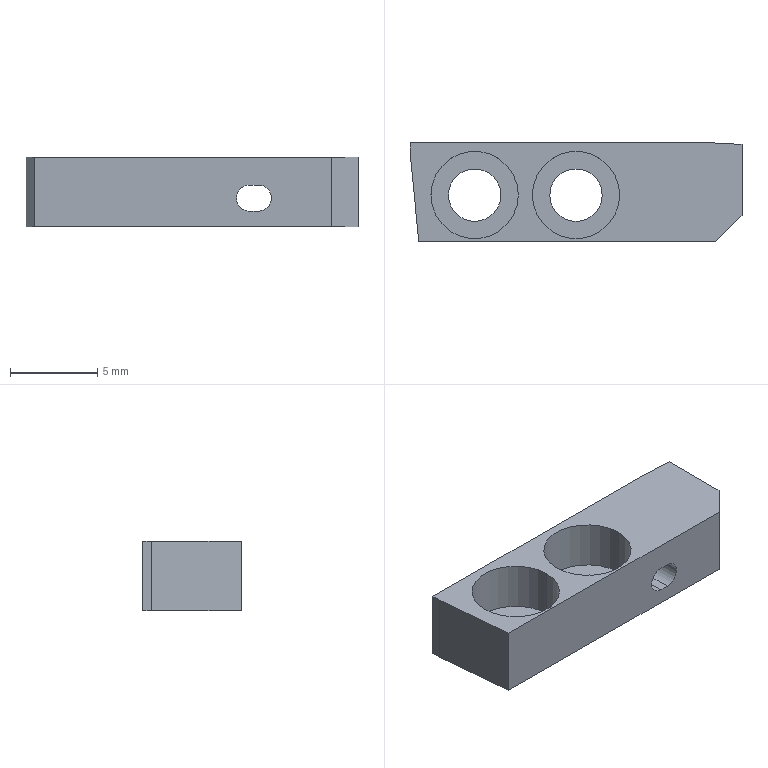Part | NX | 1 solid | 24 faces | box 19 x 5.65 x 4 mm | volume 278.189 mm3 | plane 13 | cylinder 11 | commonest cylinder face diameters 3 x4 5 x4 1.5 x3
STEP:
#1=CARTESIAN_POINT('',(1.2,2.65,4.));
#2=VERTEX_POINT('',#1);
#3=CARTESIAN_POINT('',(6.2,2.65,4.));
#4=VERTEX_POINT('',#3);
#5=CARTESIAN_POINT('',(3.7,2.65,4.));
#6=DIRECTION('',(0.,0.,1.));
#7=DIRECTION('',(1.,0.,0.));
#8=AXIS2_PLACEMENT_3D('',#5,#6,#7);
#9=CIRCLE('',#8,2.5);
#10=EDGE_CURVE('',#2,#4,#9,.T.);
#11=ORIENTED_EDGE('',*,*,#10,.T.);
#12=CARTESIAN_POINT('',(6.2,2.65,1.2));
#13=VERTEX_POINT('',#12);
#14=CARTESIAN_POINT('',(6.2,2.65,4.));
#15=DIRECTION('',(0.,0.,1.));
#16=VECTOR('',#15,1000.);
#17=LINE('',#14,#16);
#18=EDGE_CURVE('',#13,#4,#17,.T.);
#19=ORIENTED_EDGE('',*,*,#18,.F.);
#20=CARTESIAN_POINT('',(1.2,2.65,1.2));
#21=VERTEX_POINT('',#20);
#22=CARTESIAN_POINT('',(3.7,2.65,1.2));
#23=DIRECTION('',(0.,0.,1.));
#24=DIRECTION('',(1.,0.,0.));
#25=AXIS2_PLACEMENT_3D('',#22,#23,#24);
#26=CIRCLE('',#25,2.5);
#27=EDGE_CURVE('',#21,#13,#26,.T.);
#28=ORIENTED_EDGE('',*,*,#27,.F.);
#29=CARTESIAN_POINT('',(1.2,2.65,4.));
#30=DIRECTION('',(0.,0.,1.));
#31=VECTOR('',#30,1000.);
#32=LINE('',#29,#31);
#33=EDGE_CURVE('',#21,#2,#32,.T.);
#34=ORIENTED_EDGE('',*,*,#33,.T.);
#35=EDGE_LOOP('',(#11,#19,#28,#34));
#36=FACE_BOUND('',#35,.T.);
#37=CARTESIAN_POINT('',(3.7,2.65,4.));
#38=DIRECTION('',(0.,0.,1.));
#39=DIRECTION('',(1.,0.,0.));
#40=AXIS2_PLACEMENT_3D('',#37,#38,#39);
#41=CYLINDRICAL_SURFACE('',#40,2.5);
#42=ADVANCED_FACE('',(#36),#41,.F.);
#43=CARTESIAN_POINT('',(17.,5.65,0.));
#44=VERTEX_POINT('',#43);
#45=CARTESIAN_POINT('',(0.,5.65,0.));
#46=VERTEX_POINT('',#45);
#47=CARTESIAN_POINT('',(0.,5.65,0.));
#48=DIRECTION('',(-1.,0.,0.));
#49=VECTOR('',#48,1000.);
#50=LINE('',#47,#49);
#51=EDGE_CURVE('',#44,#46,#50,.T.);
#52=ORIENTED_EDGE('',*,*,#51,.T.);
#53=CARTESIAN_POINT('',(0.,5.65,4.));
#54=VERTEX_POINT('',#53);
#55=CARTESIAN_POINT('',(0.,5.65,0.));
#56=DIRECTION('',(0.,0.,1.));
#57=VECTOR('',#56,1000.);
#58=LINE('',#55,#57);
#59=EDGE_CURVE('',#46,#54,#58,.T.);
#60=ORIENTED_EDGE('',*,*,#59,.T.);
#61=CARTESIAN_POINT('',(17.,5.65,4.));
#62=VERTEX_POINT('',#61);
#63=CARTESIAN_POINT('',(0.,5.65,4.));
#64=DIRECTION('',(-1.,0.,0.));
#65=VECTOR('',#64,1000.);
#66=LINE('',#63,#65);
#67=EDGE_CURVE('',#62,#54,#66,.T.);
#68=ORIENTED_EDGE('',*,*,#67,.F.);
#69=CARTESIAN_POINT('',(17.,5.65,0.));
#70=DIRECTION('',(0.,0.,1.));
#71=VECTOR('',#70,1000.);
#72=LINE('',#69,#71);
#73=EDGE_CURVE('',#44,#62,#72,.T.);
#74=ORIENTED_EDGE('',*,*,#73,.F.);
#75=EDGE_LOOP('',(#52,#60,#68,#74));
#76=FACE_BOUND('',#75,.T.);
#77=CARTESIAN_POINT('',(12.8,5.65,0.9));
#78=VERTEX_POINT('',#77);
#79=CARTESIAN_POINT('',(13.3,5.65,0.9));
#80=VERTEX_POINT('',#79);
#81=CARTESIAN_POINT('',(0.,5.65,0.9));
#82=DIRECTION('',(1.,0.,0.));
#83=VECTOR('',#82,1000.);
#84=LINE('',#81,#83);
#85=EDGE_CURVE('',#78,#80,#84,.T.);
#86=ORIENTED_EDGE('',*,*,#85,.T.);
#87=CARTESIAN_POINT('',(13.3,5.65,2.4));
#88=VERTEX_POINT('',#87);
#89=CARTESIAN_POINT('',(13.3,5.65,1.65));
#90=DIRECTION('',(0.,1.,0.));
#91=DIRECTION('',(-1.,0.,0.));
#92=AXIS2_PLACEMENT_3D('',#89,#90,#91);
#93=CIRCLE('',#92,0.75);
#94=EDGE_CURVE('',#88,#80,#93,.T.);
#95=ORIENTED_EDGE('',*,*,#94,.F.);
#96=CARTESIAN_POINT('',(12.8,5.65,2.4));
#97=VERTEX_POINT('',#96);
#98=CARTESIAN_POINT('',(0.,5.65,2.4));
#99=DIRECTION('',(-1.,0.,0.));
#100=VECTOR('',#99,1000.);
#101=LINE('',#98,#100);
#102=EDGE_CURVE('',#88,#97,#101,.T.);
#103=ORIENTED_EDGE('',*,*,#102,.T.);
#104=CARTESIAN_POINT('',(12.05,5.65,1.65));
#105=VERTEX_POINT('',#104);
#106=CARTESIAN_POINT('',(12.8,5.65,1.65));
#107=DIRECTION('',(0.,1.,0.));
#108=DIRECTION('',(-1.,0.,0.));
#109=AXIS2_PLACEMENT_3D('',#106,#107,#108);
#110=CIRCLE('',#109,0.75);
#111=EDGE_CURVE('',#105,#97,#110,.T.);
#112=ORIENTED_EDGE('',*,*,#111,.F.);
#113=CARTESIAN_POINT('',(12.8,5.65,1.65));
#114=DIRECTION('',(0.,1.,0.));
#115=DIRECTION('',(-1.,0.,0.));
#116=AXIS2_PLACEMENT_3D('',#113,#114,#115);
#117=CIRCLE('',#116,0.75);
#118=EDGE_CURVE('',#78,#105,#117,.T.);
#119=ORIENTED_EDGE('',*,*,#118,.F.);
#120=EDGE_LOOP('',(#86,#95,#103,#112,#119));
#121=FACE_BOUND('',#120,.T.);
#122=CARTESIAN_POINT('',(19.,5.65,0.));
#123=DIRECTION('',(0.,1.,0.));
#124=DIRECTION('',(1.,0.,0.));
#125=AXIS2_PLACEMENT_3D('',#122,#123,#124);
#126=PLANE('',#125);
#127=ADVANCED_FACE('',(#76,#121),#126,.T.);
#128=CARTESIAN_POINT('',(0.,5.15,4.));
#129=VERTEX_POINT('',#128);
#130=CARTESIAN_POINT('',(0.,5.15,0.));
#131=VERTEX_POINT('',#130);
#132=CARTESIAN_POINT('',(0.,5.15,0.));
#133=DIRECTION('',(0.,0.,-1.));
#134=VECTOR('',#133,1000.);
#135=LINE('',#132,#134);
#136=EDGE_CURVE('',#129,#131,#135,.T.);
#137=ORIENTED_EDGE('',*,*,#136,.F.);
#138=CARTESIAN_POINT('',(0.,0.,4.));
#139=DIRECTION('',(0.,-1.,0.));
#140=VECTOR('',#139,1000.);
#141=LINE('',#138,#140);
#142=EDGE_CURVE('',#54,#129,#141,.T.);
#143=ORIENTED_EDGE('',*,*,#142,.F.);
#144=ORIENTED_EDGE('',*,*,#59,.F.);
#145=CARTESIAN_POINT('',(0.,0.,0.));
#146=DIRECTION('',(0.,-1.,0.));
#147=VECTOR('',#146,1000.);
#148=LINE('',#145,#147);
#149=EDGE_CURVE('',#46,#131,#148,.T.);
#150=ORIENTED_EDGE('',*,*,#149,.T.);
#151=EDGE_LOOP('',(#137,#143,#144,#150));
#152=FACE_BOUND('',#151,.T.);
#153=CARTESIAN_POINT('',(0.,5.65,0.));
#154=DIRECTION('',(-1.,0.,0.));
#155=DIRECTION('',(0.,0.,1.));
#156=AXIS2_PLACEMENT_3D('',#153,#154,#155);
#157=PLANE('',#156);
#158=ADVANCED_FACE('',(#152),#157,.T.);
#159=CARTESIAN_POINT('',(12.,2.65,1.2));
#160=VERTEX_POINT('',#159);
#161=CARTESIAN_POINT('',(7.,2.65,1.2));
#162=VERTEX_POINT('',#161);
#163=CARTESIAN_POINT('',(9.5,2.65,1.2));
#164=DIRECTION('',(0.,0.,1.));
#165=DIRECTION('',(-1.,0.,0.));
#166=AXIS2_PLACEMENT_3D('',#163,#164,#165);
#167=CIRCLE('',#166,2.5);
#168=EDGE_CURVE('',#160,#162,#167,.T.);
#169=ORIENTED_EDGE('',*,*,#168,.T.);
#170=CARTESIAN_POINT('',(9.5,2.65,1.2));
#171=DIRECTION('',(0.,0.,1.));
#172=DIRECTION('',(-1.,0.,0.));
#173=AXIS2_PLACEMENT_3D('',#170,#171,#172);
#174=CIRCLE('',#173,2.5);
#175=EDGE_CURVE('',#162,#160,#174,.T.);
#176=ORIENTED_EDGE('',*,*,#175,.T.);
#177=EDGE_LOOP('',(#169,#176));
#178=FACE_BOUND('',#177,.T.);
#179=CARTESIAN_POINT('',(11.,2.65,1.2));
#180=VERTEX_POINT('',#179);
#181=CARTESIAN_POINT('',(8.,2.65,1.2));
#182=VERTEX_POINT('',#181);
#183=CARTESIAN_POINT('',(9.5,2.65,1.2));
#184=DIRECTION('',(0.,0.,1.));
#185=DIRECTION('',(-1.,0.,0.));
#186=AXIS2_PLACEMENT_3D('',#183,#184,#185);
#187=CIRCLE('',#186,1.5);
#188=EDGE_CURVE('',#180,#182,#187,.T.);
#189=ORIENTED_EDGE('',*,*,#188,.F.);
#190=CARTESIAN_POINT('',(9.5,2.65,1.2));
#191=DIRECTION('',(0.,0.,1.));
#192=DIRECTION('',(-1.,0.,0.));
#193=AXIS2_PLACEMENT_3D('',#190,#191,#192);
#194=CIRCLE('',#193,1.5);
#195=EDGE_CURVE('',#182,#180,#194,.T.);
#196=ORIENTED_EDGE('',*,*,#195,.F.);
#197=EDGE_LOOP('',(#189,#196));
#198=FACE_BOUND('',#197,.T.);
#199=CARTESIAN_POINT('',(9.5,2.65,1.2));
#200=DIRECTION('',(0.,0.,1.));
#201=DIRECTION('',(1.,0.,0.));
#202=AXIS2_PLACEMENT_3D('',#199,#200,#201);
#203=PLANE('',#202);
#204=ADVANCED_FACE('',(#178,#198),#203,.T.);
#205=ORIENTED_EDGE('',*,*,#73,.T.);
#206=CARTESIAN_POINT('',(19.,5.545,4.));
#207=VERTEX_POINT('',#206);
#208=CARTESIAN_POINT('',(0.,6.541,4.));
#209=DIRECTION('',(-0.9986,0.05234,0.));
#210=VECTOR('',#209,1000.);
#211=LINE('',#208,#210);
#212=EDGE_CURVE('',#207,#62,#211,.T.);
#213=ORIENTED_EDGE('',*,*,#212,.F.);
#214=CARTESIAN_POINT('',(19.,5.545,0.));
#215=VERTEX_POINT('',#214);
#216=CARTESIAN_POINT('',(19.,5.545,0.));
#217=DIRECTION('',(0.,0.,-1.));
#218=VECTOR('',#217,1000.);
#219=LINE('',#216,#218);
#220=EDGE_CURVE('',#207,#215,#219,.T.);
#221=ORIENTED_EDGE('',*,*,#220,.T.);
#222=CARTESIAN_POINT('',(0.,6.541,0.));
#223=DIRECTION('',(-0.9986,0.05234,0.));
#224=VECTOR('',#223,1000.);
#225=LINE('',#222,#224);
#226=EDGE_CURVE('',#215,#44,#225,.T.);
#227=ORIENTED_EDGE('',*,*,#226,.T.);
#228=EDGE_LOOP('',(#205,#213,#221,#227));
#229=FACE_BOUND('',#228,.T.);
#230=CARTESIAN_POINT('',(17.,5.65,0.));
#231=DIRECTION('',(0.05234,0.9986,0.));
#232=DIRECTION('',(0.,0.,-1.));
#233=AXIS2_PLACEMENT_3D('',#230,#231,#232);
#234=PLANE('',#233);
#235=ADVANCED_FACE('',(#229),#234,.T.);
#236=CARTESIAN_POINT('',(19.,1.5,0.));
#237=VERTEX_POINT('',#236);
#238=CARTESIAN_POINT('',(19.,0.,0.));
#239=DIRECTION('',(0.,1.,0.));
#240=VECTOR('',#239,1000.);
#241=LINE('',#238,#240);
#242=EDGE_CURVE('',#237,#215,#241,.T.);
#243=ORIENTED_EDGE('',*,*,#242,.T.);
#244=ORIENTED_EDGE('',*,*,#220,.F.);
#245=CARTESIAN_POINT('',(19.,1.5,4.));
#246=VERTEX_POINT('',#245);
#247=CARTESIAN_POINT('',(19.,0.,4.));
#248=DIRECTION('',(0.,1.,0.));
#249=VECTOR('',#248,1000.);
#250=LINE('',#247,#249);
#251=EDGE_CURVE('',#246,#207,#250,.T.);
#252=ORIENTED_EDGE('',*,*,#251,.F.);
#253=CARTESIAN_POINT('',(19.,1.5,0.));
#254=DIRECTION('',(0.,0.,1.));
#255=VECTOR('',#254,1000.);
#256=LINE('',#253,#255);
#257=EDGE_CURVE('',#237,#246,#256,.T.);
#258=ORIENTED_EDGE('',*,*,#257,.F.);
#259=EDGE_LOOP('',(#243,#244,#252,#258));
#260=FACE_BOUND('',#259,.T.);
#261=CARTESIAN_POINT('',(19.,0.,0.));
#262=DIRECTION('',(1.,0.,0.));
#263=DIRECTION('',(0.,1.,0.));
#264=AXIS2_PLACEMENT_3D('',#261,#262,#263);
#265=PLANE('',#264);
#266=ADVANCED_FACE('',(#260),#265,.T.);
#267=ORIENTED_EDGE('',*,*,#257,.T.);
#268=CARTESIAN_POINT('',(17.5,0.,4.));
#269=VERTEX_POINT('',#268);
#270=CARTESIAN_POINT('',(17.5,0.,4.));
#271=DIRECTION('',(0.7071,0.7071,0.));
#272=VECTOR('',#271,1000.);
#273=LINE('',#270,#272);
#274=EDGE_CURVE('',#269,#246,#273,.T.);
#275=ORIENTED_EDGE('',*,*,#274,.F.);
#276=CARTESIAN_POINT('',(17.5,0.,0.));
#277=VERTEX_POINT('',#276);
#278=CARTESIAN_POINT('',(17.5,0.,0.));
#279=DIRECTION('',(0.,0.,1.));
#280=VECTOR('',#279,1000.);
#281=LINE('',#278,#280);
#282=EDGE_CURVE('',#277,#269,#281,.T.);
#283=ORIENTED_EDGE('',*,*,#282,.F.);
#284=CARTESIAN_POINT('',(17.5,0.,0.));
#285=DIRECTION('',(0.7071,0.7071,0.));
#286=VECTOR('',#285,1000.);
#287=LINE('',#284,#286);
#288=EDGE_CURVE('',#277,#237,#287,.T.);
#289=ORIENTED_EDGE('',*,*,#288,.T.);
#290=EDGE_LOOP('',(#267,#275,#283,#289));
#291=FACE_BOUND('',#290,.T.);
#292=CARTESIAN_POINT('',(19.,1.5,0.));
#293=DIRECTION('',(0.7071,-0.7071,0.));
#294=DIRECTION('',(0.,0.,-1.));
#295=AXIS2_PLACEMENT_3D('',#292,#293,#294);
#296=PLANE('',#295);
#297=ADVANCED_FACE('',(#291),#296,.T.);
#298=CARTESIAN_POINT('',(3.7,2.65,1.2));
#299=DIRECTION('',(0.,0.,1.));
#300=DIRECTION('',(1.,0.,0.));
#301=AXIS2_PLACEMENT_3D('',#298,#299,#300);
#302=CIRCLE('',#301,2.5);
#303=EDGE_CURVE('',#13,#21,#302,.T.);
#304=ORIENTED_EDGE('',*,*,#303,.T.);
#305=ORIENTED_EDGE('',*,*,#27,.T.);
#306=EDGE_LOOP('',(#304,#305));
#307=FACE_BOUND('',#306,.T.);
#308=CARTESIAN_POINT('',(5.2,2.65,1.2));
#309=VERTEX_POINT('',#308);
#310=CARTESIAN_POINT('',(2.2,2.65,1.2));
#311=VERTEX_POINT('',#310);
#312=CARTESIAN_POINT('',(3.7,2.65,1.2));
#313=DIRECTION('',(0.,0.,1.));
#314=DIRECTION('',(-1.,0.,0.));
#315=AXIS2_PLACEMENT_3D('',#312,#313,#314);
#316=CIRCLE('',#315,1.5);
#317=EDGE_CURVE('',#309,#311,#316,.T.);
#318=ORIENTED_EDGE('',*,*,#317,.F.);
#319=CARTESIAN_POINT('',(3.7,2.65,1.2));
#320=DIRECTION('',(0.,0.,1.));
#321=DIRECTION('',(-1.,0.,0.));
#322=AXIS2_PLACEMENT_3D('',#319,#320,#321);
#323=CIRCLE('',#322,1.5);
#324=EDGE_CURVE('',#311,#309,#323,.T.);
#325=ORIENTED_EDGE('',*,*,#324,.F.);
#326=EDGE_LOOP('',(#318,#325));
#327=FACE_BOUND('',#326,.T.);
#328=CARTESIAN_POINT('',(8.521,3.606,1.2));
#329=DIRECTION('',(0.,0.,1.));
#330=DIRECTION('',(1.,0.,0.));
#331=AXIS2_PLACEMENT_3D('',#328,#329,#330);
#332=PLANE('',#331);
#333=ADVANCED_FACE('',(#307,#327),#332,.T.);
#334=CARTESIAN_POINT('',(12.,2.65,4.));
#335=VERTEX_POINT('',#334);
#336=CARTESIAN_POINT('',(7.,2.65,4.));
#337=VERTEX_POINT('',#336);
#338=CARTESIAN_POINT('',(9.5,2.65,4.));
#339=DIRECTION('',(0.,0.,1.));
#340=DIRECTION('',(-1.,0.,0.));
#341=AXIS2_PLACEMENT_3D('',#338,#339,#340);
#342=CIRCLE('',#341,2.5);
#343=EDGE_CURVE('',#335,#337,#342,.T.);
#344=ORIENTED_EDGE('',*,*,#343,.T.);
#345=CARTESIAN_POINT('',(7.,2.65,-0.62));
#346=DIRECTION('',(0.,0.,1.));
#347=VECTOR('',#346,1000.);
#348=LINE('',#345,#347);
#349=EDGE_CURVE('',#337,#162,#348,.F.);
#350=ORIENTED_EDGE('',*,*,#349,.T.);
#351=ORIENTED_EDGE('',*,*,#168,.F.);
#352=CARTESIAN_POINT('',(12.,2.65,-0.62));
#353=DIRECTION('',(0.,0.,1.));
#354=VECTOR('',#353,1000.);
#355=LINE('',#352,#354);
#356=EDGE_CURVE('',#335,#160,#355,.F.);
#357=ORIENTED_EDGE('',*,*,#356,.F.);
#358=EDGE_LOOP('',(#344,#350,#351,#357));
#359=FACE_BOUND('',#358,.T.);
#360=CARTESIAN_POINT('',(9.5,2.65,-0.62));
#361=DIRECTION('',(0.,0.,1.));
#362=DIRECTION('',(-1.,0.,0.));
#363=AXIS2_PLACEMENT_3D('',#360,#361,#362);
#364=CYLINDRICAL_SURFACE('',#363,2.5);
#365=ADVANCED_FACE('',(#359),#364,.F.);
#366=ORIENTED_EDGE('',*,*,#317,.T.);
#367=CARTESIAN_POINT('',(2.2,2.65,0.));
#368=VERTEX_POINT('',#367);
#369=CARTESIAN_POINT('',(2.2,2.65,-0.62));
#370=DIRECTION('',(0.,0.,1.));
#371=VECTOR('',#370,1000.);
#372=LINE('',#369,#371);
#373=EDGE_CURVE('',#311,#368,#372,.F.);
#374=ORIENTED_EDGE('',*,*,#373,.T.);
#375=CARTESIAN_POINT('',(5.2,2.65,0.));
#376=VERTEX_POINT('',#375);
#377=CARTESIAN_POINT('',(3.7,2.65,0.));
#378=DIRECTION('',(0.,0.,1.));
#379=DIRECTION('',(-1.,0.,0.));
#380=AXIS2_PLACEMENT_3D('',#377,#378,#379);
#381=CIRCLE('',#380,1.5);
#382=EDGE_CURVE('',#376,#368,#381,.T.);
#383=ORIENTED_EDGE('',*,*,#382,.F.);
#384=CARTESIAN_POINT('',(5.2,2.65,-0.62));
#385=DIRECTION('',(0.,0.,1.));
#386=VECTOR('',#385,1000.);
#387=LINE('',#384,#386);
#388=EDGE_CURVE('',#309,#376,#387,.F.);
#389=ORIENTED_EDGE('',*,*,#388,.F.);
#390=EDGE_LOOP('',(#366,#374,#383,#389));
#391=FACE_BOUND('',#390,.T.);
#392=CARTESIAN_POINT('',(3.7,2.65,-0.62));
#393=DIRECTION('',(0.,0.,1.));
#394=DIRECTION('',(-1.,0.,0.));
#395=AXIS2_PLACEMENT_3D('',#392,#393,#394);
#396=CYLINDRICAL_SURFACE('',#395,1.5);
#397=ADVANCED_FACE('',(#391),#396,.F.);
#398=ORIENTED_EDGE('',*,*,#149,.F.);
#399=ORIENTED_EDGE('',*,*,#51,.F.);
#400=ORIENTED_EDGE('',*,*,#226,.F.);
#401=ORIENTED_EDGE('',*,*,#242,.F.);
#402=ORIENTED_EDGE('',*,*,#288,.F.);
#403=CARTESIAN_POINT('',(0.5,0.,0.));
#404=VERTEX_POINT('',#403);
#405=CARTESIAN_POINT('',(0.,0.,0.));
#406=DIRECTION('',(1.,0.,0.));
#407=VECTOR('',#406,1000.);
#408=LINE('',#405,#407);
#409=EDGE_CURVE('',#404,#277,#408,.T.);
#410=ORIENTED_EDGE('',*,*,#409,.F.);
#411=CARTESIAN_POINT('',(0.5,0.,0.));
#412=DIRECTION('',(-0.09663,0.9953,0.));
#413=VECTOR('',#412,1000.);
#414=LINE('',#411,#413);
#415=EDGE_CURVE('',#404,#131,#414,.T.);
#416=ORIENTED_EDGE('',*,*,#415,.T.);
#417=EDGE_LOOP('',(#398,#399,#400,#401,#402,#410,#416));
#418=FACE_BOUND('',#417,.T.);
#419=CARTESIAN_POINT('',(11.,2.65,0.));
#420=VERTEX_POINT('',#419);
#421=CARTESIAN_POINT('',(8.,2.65,0.));
#422=VERTEX_POINT('',#421);
#423=CARTESIAN_POINT('',(9.5,2.65,0.));
#424=DIRECTION('',(0.,0.,1.));
#425=DIRECTION('',(-1.,0.,0.));
#426=AXIS2_PLACEMENT_3D('',#423,#424,#425);
#427=CIRCLE('',#426,1.5);
#428=EDGE_CURVE('',#420,#422,#427,.T.);
#429=ORIENTED_EDGE('',*,*,#428,.T.);
#430=CARTESIAN_POINT('',(9.5,2.65,0.));
#431=DIRECTION('',(0.,0.,1.));
#432=DIRECTION('',(-1.,0.,0.));
#433=AXIS2_PLACEMENT_3D('',#430,#431,#432);
#434=CIRCLE('',#433,1.5);
#435=EDGE_CURVE('',#422,#420,#434,.T.);
#436=ORIENTED_EDGE('',*,*,#435,.T.);
#437=EDGE_LOOP('',(#429,#436));
#438=FACE_BOUND('',#437,.T.);
#439=CARTESIAN_POINT('',(3.7,2.65,0.));
#440=DIRECTION('',(0.,0.,1.));
#441=DIRECTION('',(-1.,0.,0.));
#442=AXIS2_PLACEMENT_3D('',#439,#440,#441);
#443=CIRCLE('',#442,1.5);
#444=EDGE_CURVE('',#368,#376,#443,.T.);
#445=ORIENTED_EDGE('',*,*,#444,.T.);
#446=ORIENTED_EDGE('',*,*,#382,.T.);
#447=EDGE_LOOP('',(#445,#446));
#448=FACE_BOUND('',#447,.T.);
#449=CARTESIAN_POINT('',(0.,0.,0.));
#450=DIRECTION('',(0.,0.,1.));
#451=DIRECTION('',(1.,0.,0.));
#452=AXIS2_PLACEMENT_3D('',#449,#450,#451);
#453=PLANE('',#452);
#454=ADVANCED_FACE('',(#418,#438,#448),#453,.F.);
#455=ORIENTED_EDGE('',*,*,#188,.T.);
#456=CARTESIAN_POINT('',(8.,2.65,-0.62));
#457=DIRECTION('',(0.,0.,1.));
#458=VECTOR('',#457,1000.);
#459=LINE('',#456,#458);
#460=EDGE_CURVE('',#182,#422,#459,.F.);
#461=ORIENTED_EDGE('',*,*,#460,.T.);
#462=ORIENTED_EDGE('',*,*,#428,.F.);
#463=CARTESIAN_POINT('',(11.,2.65,-0.62));
#464=DIRECTION('',(0.,0.,1.));
#465=VECTOR('',#464,1000.);
#466=LINE('',#463,#465);
#467=EDGE_CURVE('',#180,#420,#466,.F.);
#468=ORIENTED_EDGE('',*,*,#467,.F.);
#469=EDGE_LOOP('',(#455,#461,#462,#468));
#470=FACE_BOUND('',#469,.T.);
#471=CARTESIAN_POINT('',(9.5,2.65,-0.62));
#472=DIRECTION('',(0.,0.,1.));
#473=DIRECTION('',(-1.,0.,0.));
#474=AXIS2_PLACEMENT_3D('',#471,#472,#473);
#475=CYLINDRICAL_SURFACE('',#474,1.5);
#476=ADVANCED_FACE('',(#470),#475,.F.);
#477=CARTESIAN_POINT('',(0.5,0.,4.));
#478=VERTEX_POINT('',#477);
#479=CARTESIAN_POINT('',(0.,0.,4.));
#480=DIRECTION('',(-1.,0.,0.));
#481=VECTOR('',#480,1000.);
#482=LINE('',#479,#481);
#483=EDGE_CURVE('',#269,#478,#482,.T.);
#484=ORIENTED_EDGE('',*,*,#483,.F.);
#485=ORIENTED_EDGE('',*,*,#274,.T.);
#486=ORIENTED_EDGE('',*,*,#251,.T.);
#487=ORIENTED_EDGE('',*,*,#212,.T.);
#488=ORIENTED_EDGE('',*,*,#67,.T.);
#489=ORIENTED_EDGE('',*,*,#142,.T.);
#490=CARTESIAN_POINT('',(0.5,0.,4.));
#491=DIRECTION('',(-0.09663,0.9953,0.));
#492=VECTOR('',#491,1000.);
#493=LINE('',#490,#492);
#494=EDGE_CURVE('',#478,#129,#493,.T.);
#495=ORIENTED_EDGE('',*,*,#494,.F.);
#496=EDGE_LOOP('',(#484,#485,#486,#487,#488,#489,#495));
#497=FACE_BOUND('',#496,.T.);
#498=ORIENTED_EDGE('',*,*,#343,.F.);
#499=CARTESIAN_POINT('',(9.5,2.65,4.));
#500=DIRECTION('',(0.,0.,1.));
#501=DIRECTION('',(-1.,0.,0.));
#502=AXIS2_PLACEMENT_3D('',#499,#500,#501);
#503=CIRCLE('',#502,2.5);
#504=EDGE_CURVE('',#337,#335,#503,.T.);
#505=ORIENTED_EDGE('',*,*,#504,.F.);
#506=EDGE_LOOP('',(#498,#505));
#507=FACE_BOUND('',#506,.T.);
#508=ORIENTED_EDGE('',*,*,#10,.F.);
#509=CARTESIAN_POINT('',(3.7,2.65,4.));
#510=DIRECTION('',(0.,0.,1.));
#511=DIRECTION('',(1.,0.,0.));
#512=AXIS2_PLACEMENT_3D('',#509,#510,#511);
#513=CIRCLE('',#512,2.5);
#514=EDGE_CURVE('',#4,#2,#513,.T.);
#515=ORIENTED_EDGE('',*,*,#514,.F.);
#516=EDGE_LOOP('',(#508,#515));
#517=FACE_BOUND('',#516,.T.);
#518=CARTESIAN_POINT('',(0.,0.,4.));
#519=DIRECTION('',(0.,0.,1.));
#520=DIRECTION('',(1.,0.,0.));
#521=AXIS2_PLACEMENT_3D('',#518,#519,#520);
#522=PLANE('',#521);
#523=ADVANCED_FACE('',(#497,#507,#517),#522,.T.);
#524=CARTESIAN_POINT('',(0.5,0.,0.));
#525=DIRECTION('',(0.,0.,1.));
#526=VECTOR('',#525,1000.);
#527=LINE('',#524,#526);
#528=EDGE_CURVE('',#404,#478,#527,.T.);
#529=ORIENTED_EDGE('',*,*,#528,.F.);
#530=ORIENTED_EDGE('',*,*,#409,.T.);
#531=ORIENTED_EDGE('',*,*,#282,.T.);
#532=ORIENTED_EDGE('',*,*,#483,.T.);
#533=EDGE_LOOP('',(#529,#530,#531,#532));
#534=FACE_BOUND('',#533,.T.);
#535=CARTESIAN_POINT('',(13.3,0.,0.9));
#536=VERTEX_POINT('',#535);
#537=CARTESIAN_POINT('',(12.8,0.,0.9));
#538=VERTEX_POINT('',#537);
#539=CARTESIAN_POINT('',(0.,0.,0.9));
#540=DIRECTION('',(-1.,0.,0.));
#541=VECTOR('',#540,1000.);
#542=LINE('',#539,#541);
#543=EDGE_CURVE('',#536,#538,#542,.T.);
#544=ORIENTED_EDGE('',*,*,#543,.T.);
#545=CARTESIAN_POINT('',(12.05,0.,1.65));
#546=VERTEX_POINT('',#545);
#547=CARTESIAN_POINT('',(12.8,0.,1.65));
#548=DIRECTION('',(0.,1.,0.));
#549=DIRECTION('',(-1.,0.,0.));
#550=AXIS2_PLACEMENT_3D('',#547,#548,#549);
#551=CIRCLE('',#550,0.75);
#552=EDGE_CURVE('',#538,#546,#551,.T.);
#553=ORIENTED_EDGE('',*,*,#552,.T.);
#554=CARTESIAN_POINT('',(12.8,0.,2.4));
#555=VERTEX_POINT('',#554);
#556=CARTESIAN_POINT('',(12.8,0.,1.65));
#557=DIRECTION('',(0.,1.,0.));
#558=DIRECTION('',(-1.,0.,0.));
#559=AXIS2_PLACEMENT_3D('',#556,#557,#558);
#560=CIRCLE('',#559,0.75);
#561=EDGE_CURVE('',#546,#555,#560,.T.);
#562=ORIENTED_EDGE('',*,*,#561,.T.);
#563=CARTESIAN_POINT('',(13.3,0.,2.4));
#564=VERTEX_POINT('',#563);
#565=CARTESIAN_POINT('',(0.,0.,2.4));
#566=DIRECTION('',(1.,0.,0.));
#567=VECTOR('',#566,1000.);
#568=LINE('',#565,#567);
#569=EDGE_CURVE('',#555,#564,#568,.T.);
#570=ORIENTED_EDGE('',*,*,#569,.T.);
#571=CARTESIAN_POINT('',(13.3,0.,1.65));
#572=DIRECTION('',(0.,1.,0.));
#573=DIRECTION('',(-1.,0.,0.));
#574=AXIS2_PLACEMENT_3D('',#571,#572,#573);
#575=CIRCLE('',#574,0.75);
#576=EDGE_CURVE('',#564,#536,#575,.T.);
#577=ORIENTED_EDGE('',*,*,#576,.T.);
#578=EDGE_LOOP('',(#544,#553,#562,#570,#577));
#579=FACE_BOUND('',#578,.T.);
#580=CARTESIAN_POINT('',(0.,0.,0.));
#581=DIRECTION('',(0.,-1.,0.));
#582=DIRECTION('',(0.,0.,-1.));
#583=AXIS2_PLACEMENT_3D('',#580,#581,#582);
#584=PLANE('',#583);
#585=ADVANCED_FACE('',(#534,#579),#584,.T.);
#586=ORIENTED_EDGE('',*,*,#543,.F.);
#587=CARTESIAN_POINT('',(13.3,-0.5652,0.9));
#588=DIRECTION('',(0.,1.,0.));
#589=VECTOR('',#588,1000.);
#590=LINE('',#587,#589);
#591=EDGE_CURVE('',#536,#80,#590,.T.);
#592=ORIENTED_EDGE('',*,*,#591,.T.);
#593=ORIENTED_EDGE('',*,*,#85,.F.);
#594=CARTESIAN_POINT('',(12.8,-0.5652,0.9));
#595=DIRECTION('',(0.,1.,0.));
#596=VECTOR('',#595,1000.);
#597=LINE('',#594,#596);
#598=EDGE_CURVE('',#538,#78,#597,.T.);
#599=ORIENTED_EDGE('',*,*,#598,.F.);
#600=EDGE_LOOP('',(#586,#592,#593,#599));
#601=FACE_BOUND('',#600,.T.);
#602=CARTESIAN_POINT('',(12.8,-0.5652,0.9));
#603=DIRECTION('',(0.,0.,-1.));
#604=DIRECTION('',(0.,-1.,0.));
#605=AXIS2_PLACEMENT_3D('',#602,#603,#604);
#606=PLANE('',#605);
#607=ADVANCED_FACE('',(#601),#606,.F.);
#608=CARTESIAN_POINT('',(12.05,-0.5652,1.65));
#609=DIRECTION('',(0.,1.,0.));
#610=VECTOR('',#609,1000.);
#611=LINE('',#608,#610);
#612=EDGE_CURVE('',#546,#105,#611,.T.);
#613=ORIENTED_EDGE('',*,*,#612,.F.);
#614=ORIENTED_EDGE('',*,*,#552,.F.);
#615=ORIENTED_EDGE('',*,*,#598,.T.);
#616=ORIENTED_EDGE('',*,*,#118,.T.);
#617=EDGE_LOOP('',(#613,#614,#615,#616));
#618=FACE_BOUND('',#617,.T.);
#619=CARTESIAN_POINT('',(12.8,-0.5652,1.65));
#620=DIRECTION('',(0.,1.,0.));
#621=DIRECTION('',(-1.,0.,0.));
#622=AXIS2_PLACEMENT_3D('',#619,#620,#621);
#623=CYLINDRICAL_SURFACE('',#622,0.75);
#624=ADVANCED_FACE('',(#618),#623,.F.);
#625=ORIENTED_EDGE('',*,*,#102,.F.);
#626=CARTESIAN_POINT('',(13.3,-0.5652,2.4));
#627=DIRECTION('',(0.,1.,0.));
#628=VECTOR('',#627,1000.);
#629=LINE('',#626,#628);
#630=EDGE_CURVE('',#564,#88,#629,.T.);
#631=ORIENTED_EDGE('',*,*,#630,.F.);
#632=ORIENTED_EDGE('',*,*,#569,.F.);
#633=CARTESIAN_POINT('',(12.8,-0.5652,2.4));
#634=DIRECTION('',(0.,1.,0.));
#635=VECTOR('',#634,1000.);
#636=LINE('',#633,#635);
#637=EDGE_CURVE('',#555,#97,#636,.T.);
#638=ORIENTED_EDGE('',*,*,#637,.T.);
#639=EDGE_LOOP('',(#625,#631,#632,#638));
#640=FACE_BOUND('',#639,.T.);
#641=CARTESIAN_POINT('',(13.3,-0.5652,2.4));
#642=DIRECTION('',(0.,0.,1.));
#643=DIRECTION('',(1.,0.,0.));
#644=AXIS2_PLACEMENT_3D('',#641,#642,#643);
#645=PLANE('',#644);
#646=ADVANCED_FACE('',(#640),#645,.F.);
#647=ORIENTED_EDGE('',*,*,#576,.F.);
#648=ORIENTED_EDGE('',*,*,#630,.T.);
#649=ORIENTED_EDGE('',*,*,#94,.T.);
#650=ORIENTED_EDGE('',*,*,#591,.F.);
#651=EDGE_LOOP('',(#647,#648,#649,#650));
#652=FACE_BOUND('',#651,.T.);
#653=CARTESIAN_POINT('',(13.3,-0.5652,1.65));
#654=DIRECTION('',(0.,1.,0.));
#655=DIRECTION('',(-1.,0.,0.));
#656=AXIS2_PLACEMENT_3D('',#653,#654,#655);
#657=CYLINDRICAL_SURFACE('',#656,0.75);
#658=ADVANCED_FACE('',(#652),#657,.F.);
#659=ORIENTED_EDGE('',*,*,#528,.T.);
#660=ORIENTED_EDGE('',*,*,#494,.T.);
#661=ORIENTED_EDGE('',*,*,#136,.T.);
#662=ORIENTED_EDGE('',*,*,#415,.F.);
#663=EDGE_LOOP('',(#659,#660,#661,#662));
#664=FACE_BOUND('',#663,.T.);
#665=CARTESIAN_POINT('',(0.25,2.575,2.));
#666=DIRECTION('',(-0.9953,-0.09663,0.));
#667=DIRECTION('',(-0.09663,0.9953,0.));
#668=AXIS2_PLACEMENT_3D('',#665,#666,#667);
#669=PLANE('',#668);
#670=ADVANCED_FACE('',(#664),#669,.T.);
#671=ORIENTED_EDGE('',*,*,#444,.F.);
#672=ORIENTED_EDGE('',*,*,#373,.F.);
#673=ORIENTED_EDGE('',*,*,#324,.T.);
#674=ORIENTED_EDGE('',*,*,#388,.T.);
#675=EDGE_LOOP('',(#671,#672,#673,#674));
#676=FACE_BOUND('',#675,.T.);
#677=CARTESIAN_POINT('',(3.7,2.65,-0.62));
#678=DIRECTION('',(0.,0.,1.));
#679=DIRECTION('',(-1.,0.,0.));
#680=AXIS2_PLACEMENT_3D('',#677,#678,#679);
#681=CYLINDRICAL_SURFACE('',#680,1.5);
#682=ADVANCED_FACE('',(#676),#681,.F.);
#683=ORIENTED_EDGE('',*,*,#349,.F.);
#684=ORIENTED_EDGE('',*,*,#504,.T.);
#685=ORIENTED_EDGE('',*,*,#356,.T.);
#686=ORIENTED_EDGE('',*,*,#175,.F.);
#687=EDGE_LOOP('',(#683,#684,#685,#686));
#688=FACE_BOUND('',#687,.T.);
#689=CARTESIAN_POINT('',(9.5,2.65,-0.62));
#690=DIRECTION('',(0.,0.,1.));
#691=DIRECTION('',(-1.,0.,0.));
#692=AXIS2_PLACEMENT_3D('',#689,#690,#691);
#693=CYLINDRICAL_SURFACE('',#692,2.5);
#694=ADVANCED_FACE('',(#688),#693,.F.);
#695=ORIENTED_EDGE('',*,*,#303,.F.);
#696=ORIENTED_EDGE('',*,*,#18,.T.);
#697=ORIENTED_EDGE('',*,*,#514,.T.);
#698=ORIENTED_EDGE('',*,*,#33,.F.);
#699=EDGE_LOOP('',(#695,#696,#697,#698));
#700=FACE_BOUND('',#699,.T.);
#701=CARTESIAN_POINT('',(3.7,2.65,4.));
#702=DIRECTION('',(0.,0.,1.));
#703=DIRECTION('',(1.,0.,0.));
#704=AXIS2_PLACEMENT_3D('',#701,#702,#703);
#705=CYLINDRICAL_SURFACE('',#704,2.5);
#706=ADVANCED_FACE('',(#700),#705,.F.);
#707=ORIENTED_EDGE('',*,*,#460,.F.);
#708=ORIENTED_EDGE('',*,*,#195,.T.);
#709=ORIENTED_EDGE('',*,*,#467,.T.);
#710=ORIENTED_EDGE('',*,*,#435,.F.);
#711=EDGE_LOOP('',(#707,#708,#709,#710));
#712=FACE_BOUND('',#711,.T.);
#713=CARTESIAN_POINT('',(9.5,2.65,-0.62));
#714=DIRECTION('',(0.,0.,1.));
#715=DIRECTION('',(-1.,0.,0.));
#716=AXIS2_PLACEMENT_3D('',#713,#714,#715);
#717=CYLINDRICAL_SURFACE('',#716,1.5);
#718=ADVANCED_FACE('',(#712),#717,.F.);
#719=ORIENTED_EDGE('',*,*,#561,.F.);
#720=ORIENTED_EDGE('',*,*,#612,.T.);
#721=ORIENTED_EDGE('',*,*,#111,.T.);
#722=ORIENTED_EDGE('',*,*,#637,.F.);
#723=EDGE_LOOP('',(#719,#720,#721,#722));
#724=FACE_BOUND('',#723,.T.);
#725=CARTESIAN_POINT('',(12.8,-0.5652,1.65));
#726=DIRECTION('',(0.,1.,0.));
#727=DIRECTION('',(-1.,0.,0.));
#728=AXIS2_PLACEMENT_3D('',#725,#726,#727);
#729=CYLINDRICAL_SURFACE('',#728,0.75);
#730=ADVANCED_FACE('',(#724),#729,.F.);
#731=CLOSED_SHELL('',(#42,#127,#158,#204,#235,#266,#297,#333,#365,#397,#454,#476,#523,#585,#607,#624,#646,#658,#670,#682,#694,#706,#718,#730));
#732=MANIFOLD_SOLID_BREP('',#731);
#733=(LENGTH_UNIT()NAMED_UNIT(*)SI_UNIT(.MILLI.,.METRE.));
#734=UNCERTAINTY_MEASURE_WITH_UNIT(LENGTH_MEASURE(0.00001),#733,'','');
#735=(NAMED_UNIT(*)PLANE_ANGLE_UNIT()SI_UNIT($,.RADIAN.));
#736=(NAMED_UNIT(*)SI_UNIT($,.STERADIAN.)SOLID_ANGLE_UNIT());
#737=(GEOMETRIC_REPRESENTATION_CONTEXT(3)GLOBAL_UNCERTAINTY_ASSIGNED_CONTEXT((#734))GLOBAL_UNIT_ASSIGNED_CONTEXT((#733,#735,#736))REPRESENTATION_CONTEXT('',''));
#738=ADVANCED_BREP_SHAPE_REPRESENTATION('',(#732),#737);